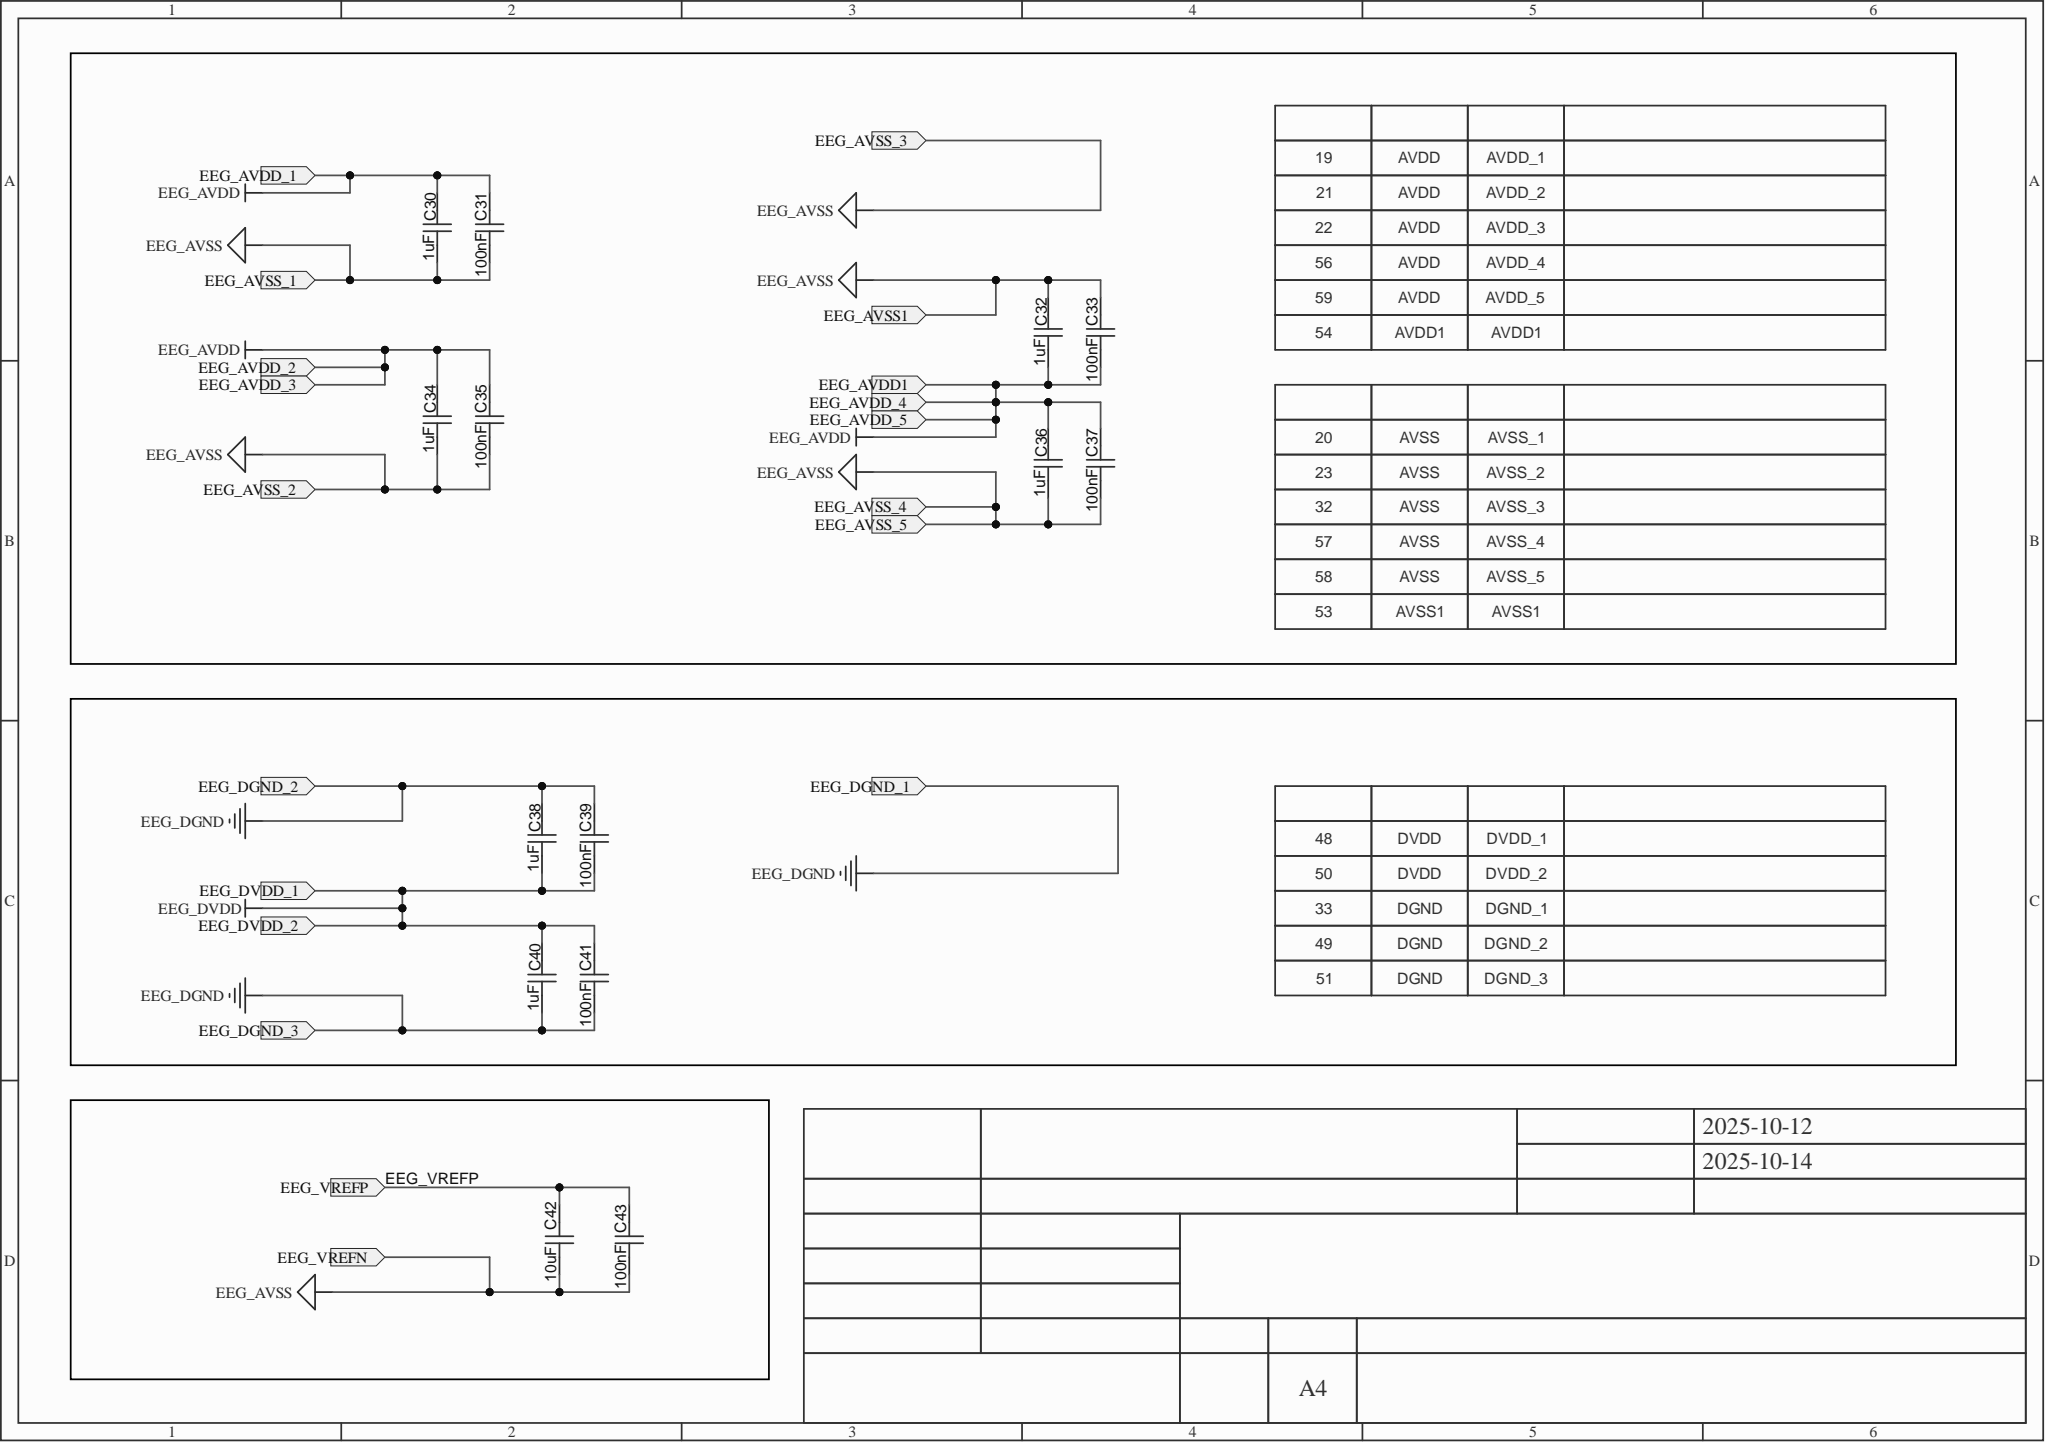Circuit board | Altium Designer | 211 parts | 126 nets | one sheet of the schematic
Parts on this sheet (reference | value | footprint):
C30 | 1uF | C0402
C31 | 100nF | C0402
C32 | 1uF | C0402
C33 | 100nF | C0402
C34 | 1uF | C0402
C35 | 100nF | C0402
C36 | 1uF | C0402
C37 | 100nF | C0402
C38 | 1uF | C0402
C39 | 100nF | C0402
C40 | 1uF | C0402
C41 | 100nF | C0402
C42 | 10uF | C0603
C43 | 100nF | C0402
Nets of these parts (net: part-pin ...):
EEG_VREFP: C42-2 C43-2
EEG_DVDD_1: C38-1 C39-1 C40-2 C41-2
EEG_DGND_1: C38-2 C39-2 C40-1 C41-1
EEG_AVSS1: C30-1 C31-1 C32-2 C33-2 C34-1 C35-1 C36-1 C37-1 C42-1 C43-1
EEG_AVDD1: C30-2 C31-2 C32-1 C33-1 C34-2 C35-2 C36-2 C37-2